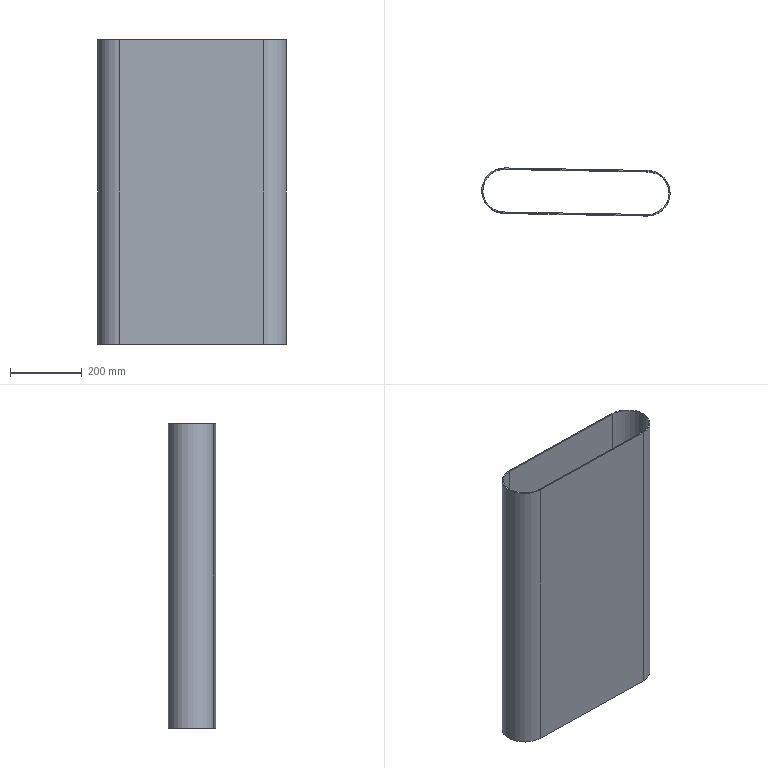Part | SolidWorks | features Extrusion 1 | 1 solid | 12 faces | box 525.939 x 132.981 x 850 mm | volume 3025361 mm3 | cylinder 6 | plane 6 | commonest cylinder face diameters 120 x3 126 x3
STEP:
#1=CARTESIAN_POINT('',(659.939,1524.019,-425.));
#2=VERTEX_POINT('',#1);
#3=CARTESIAN_POINT('',(600.986,1584.01,-425.));
#4=VERTEX_POINT('',#3);
#5=CARTESIAN_POINT('',(599.939,1524.019,-425.));
#6=DIRECTION('',(0.,0.,1.));
#7=DIRECTION('',(1.,0.,0.));
#8=AXIS2_PLACEMENT_3D('',#5,#6,#7);
#9=CIRCLE('',#8,60.);
#10=EDGE_CURVE('',#2,#4,#9,.T.);
#11=ORIENTED_EDGE('',*,*,#10,.F.);
#12=CARTESIAN_POINT('',(659.939,1524.019,425.));
#13=VERTEX_POINT('',#12);
#14=CARTESIAN_POINT('',(659.939,1524.019,-967.49));
#15=DIRECTION('',(0.,0.,1.));
#16=VECTOR('',#15,1000.);
#17=LINE('',#14,#16);
#18=EDGE_CURVE('',#2,#13,#17,.T.);
#19=ORIENTED_EDGE('',*,*,#18,.T.);
#20=CARTESIAN_POINT('',(600.986,1584.01,425.));
#21=VERTEX_POINT('',#20);
#22=CARTESIAN_POINT('',(599.939,1524.019,425.));
#23=DIRECTION('',(0.,0.,-1.));
#24=DIRECTION('',(-1.,0.,0.));
#25=AXIS2_PLACEMENT_3D('',#22,#23,#24);
#26=CIRCLE('',#25,60.);
#27=EDGE_CURVE('',#21,#13,#26,.T.);
#28=ORIENTED_EDGE('',*,*,#27,.F.);
#29=CARTESIAN_POINT('',(600.986,1584.01,-967.49));
#30=DIRECTION('',(0.,0.,1.));
#31=VECTOR('',#30,1000.);
#32=LINE('',#29,#31);
#33=EDGE_CURVE('',#4,#21,#32,.T.);
#34=ORIENTED_EDGE('',*,*,#33,.F.);
#35=EDGE_LOOP('',(#11,#19,#28,#34));
#36=FACE_OUTER_BOUND('',#35,.T.);
#37=CARTESIAN_POINT('',(599.939,1524.019,-967.49));
#38=DIRECTION('',(0.,0.,1.));
#39=DIRECTION('',(1.,0.,0.));
#40=AXIS2_PLACEMENT_3D('',#37,#38,#39);
#41=CYLINDRICAL_SURFACE('',#40,60.);
#42=ADVANCED_FACE('',(#36),#41,.F.);
#43=CARTESIAN_POINT('',(598.84,1461.029,-425.));
#44=VERTEX_POINT('',#43);
#45=CARTESIAN_POINT('',(662.939,1524.019,-425.));
#46=VERTEX_POINT('',#45);
#47=CARTESIAN_POINT('',(599.939,1524.019,-425.));
#48=DIRECTION('',(0.,0.,1.));
#49=DIRECTION('',(1.,0.,0.));
#50=AXIS2_PLACEMENT_3D('',#47,#48,#49);
#51=CIRCLE('',#50,63.);
#52=EDGE_CURVE('',#44,#46,#51,.T.);
#53=ORIENTED_EDGE('',*,*,#52,.T.);
#54=CARTESIAN_POINT('',(662.939,1524.019,425.));
#55=VERTEX_POINT('',#54);
#56=CARTESIAN_POINT('',(662.939,1524.019,-967.49));
#57=DIRECTION('',(0.,0.,1.));
#58=VECTOR('',#57,1000.);
#59=LINE('',#56,#58);
#60=EDGE_CURVE('',#46,#55,#59,.T.);
#61=ORIENTED_EDGE('',*,*,#60,.T.);
#62=CARTESIAN_POINT('',(598.84,1461.029,425.));
#63=VERTEX_POINT('',#62);
#64=CARTESIAN_POINT('',(599.939,1524.019,425.));
#65=DIRECTION('',(0.,0.,-1.));
#66=DIRECTION('',(-1.,0.,0.));
#67=AXIS2_PLACEMENT_3D('',#64,#65,#66);
#68=CIRCLE('',#67,63.);
#69=EDGE_CURVE('',#55,#63,#68,.T.);
#70=ORIENTED_EDGE('',*,*,#69,.T.);
#71=CARTESIAN_POINT('',(598.84,1461.029,-967.49));
#72=DIRECTION('',(0.,0.,1.));
#73=VECTOR('',#72,1000.);
#74=LINE('',#71,#73);
#75=EDGE_CURVE('',#44,#63,#74,.T.);
#76=ORIENTED_EDGE('',*,*,#75,.F.);
#77=EDGE_LOOP('',(#53,#61,#70,#76));
#78=FACE_OUTER_BOUND('',#77,.T.);
#79=CARTESIAN_POINT('',(599.939,1524.019,-967.49));
#80=DIRECTION('',(0.,0.,1.));
#81=DIRECTION('',(1.,0.,0.));
#82=AXIS2_PLACEMENT_3D('',#79,#80,#81);
#83=CYLINDRICAL_SURFACE('',#82,63.);
#84=ADVANCED_FACE('',(#78),#83,.T.);
#85=CARTESIAN_POINT('',(601.039,1587.009,425.));
#86=VERTEX_POINT('',#85);
#87=CARTESIAN_POINT('',(599.939,1524.019,425.));
#88=DIRECTION('',(0.,0.,-1.));
#89=DIRECTION('',(-1.,0.,0.));
#90=AXIS2_PLACEMENT_3D('',#87,#88,#89);
#91=CIRCLE('',#90,63.);
#92=EDGE_CURVE('',#86,#55,#91,.T.);
#93=ORIENTED_EDGE('',*,*,#92,.F.);
#94=CARTESIAN_POINT('',(201.1,1593.99,425.));
#95=VERTEX_POINT('',#94);
#96=CARTESIAN_POINT('',(601.039,1587.009,425.));
#97=DIRECTION('',(0.9998,-0.01745,0.));
#98=VECTOR('',#97,1000.);
#99=LINE('',#96,#98);
#100=EDGE_CURVE('',#95,#86,#99,.T.);
#101=ORIENTED_EDGE('',*,*,#100,.F.);
#102=CARTESIAN_POINT('',(198.9,1468.01,425.));
#103=VERTEX_POINT('',#102);
#104=CARTESIAN_POINT('',(200.,1531.,425.));
#105=DIRECTION('',(0.,0.,-1.));
#106=DIRECTION('',(-1.,0.,0.));
#107=AXIS2_PLACEMENT_3D('',#104,#105,#106);
#108=CIRCLE('',#107,63.);
#109=EDGE_CURVE('',#103,#95,#108,.T.);
#110=ORIENTED_EDGE('',*,*,#109,.F.);
#111=CARTESIAN_POINT('',(598.84,1461.029,425.));
#112=DIRECTION('',(-0.9998,0.01745,0.));
#113=VECTOR('',#112,1000.);
#114=LINE('',#111,#113);
#115=EDGE_CURVE('',#63,#103,#114,.T.);
#116=ORIENTED_EDGE('',*,*,#115,.F.);
#117=ORIENTED_EDGE('',*,*,#69,.F.);
#118=EDGE_LOOP('',(#93,#101,#110,#116,#117));
#119=FACE_OUTER_BOUND('',#118,.T.);
#120=ORIENTED_EDGE('',*,*,#27,.T.);
#121=CARTESIAN_POINT('',(598.892,1464.028,425.));
#122=VERTEX_POINT('',#121);
#123=CARTESIAN_POINT('',(599.939,1524.019,425.));
#124=DIRECTION('',(0.,0.,-1.));
#125=DIRECTION('',(-1.,0.,0.));
#126=AXIS2_PLACEMENT_3D('',#123,#124,#125);
#127=CIRCLE('',#126,60.);
#128=EDGE_CURVE('',#13,#122,#127,.T.);
#129=ORIENTED_EDGE('',*,*,#128,.T.);
#130=CARTESIAN_POINT('',(198.953,1471.009,425.));
#131=VERTEX_POINT('',#130);
#132=CARTESIAN_POINT('',(598.892,1464.028,425.));
#133=DIRECTION('',(-0.9998,0.01745,0.));
#134=VECTOR('',#133,1000.);
#135=LINE('',#132,#134);
#136=EDGE_CURVE('',#122,#131,#135,.T.);
#137=ORIENTED_EDGE('',*,*,#136,.T.);
#138=CARTESIAN_POINT('',(201.047,1590.991,425.));
#139=VERTEX_POINT('',#138);
#140=CARTESIAN_POINT('',(200.,1531.,425.));
#141=DIRECTION('',(0.,0.,-1.));
#142=DIRECTION('',(-1.,0.,0.));
#143=AXIS2_PLACEMENT_3D('',#140,#141,#142);
#144=CIRCLE('',#143,60.);
#145=EDGE_CURVE('',#131,#139,#144,.T.);
#146=ORIENTED_EDGE('',*,*,#145,.T.);
#147=CARTESIAN_POINT('',(600.986,1584.01,425.));
#148=DIRECTION('',(0.9998,-0.01745,0.));
#149=VECTOR('',#148,1000.);
#150=LINE('',#147,#149);
#151=EDGE_CURVE('',#139,#21,#150,.T.);
#152=ORIENTED_EDGE('',*,*,#151,.T.);
#153=EDGE_LOOP('',(#120,#129,#137,#146,#152));
#154=FACE_BOUND('',#153,.T.);
#155=CARTESIAN_POINT('',(599.939,1524.019,425.));
#156=DIRECTION('',(0.,0.,-1.));
#157=DIRECTION('',(-1.,0.,0.));
#158=AXIS2_PLACEMENT_3D('',#155,#156,#157);
#159=PLANE('',#158);
#160=ADVANCED_FACE('',(#119,#154),#159,.F.);
#161=ORIENTED_EDGE('',*,*,#60,.F.);
#162=CARTESIAN_POINT('',(601.039,1587.009,-425.));
#163=VERTEX_POINT('',#162);
#164=CARTESIAN_POINT('',(599.939,1524.019,-425.));
#165=DIRECTION('',(0.,0.,1.));
#166=DIRECTION('',(1.,0.,0.));
#167=AXIS2_PLACEMENT_3D('',#164,#165,#166);
#168=CIRCLE('',#167,63.);
#169=EDGE_CURVE('',#46,#163,#168,.T.);
#170=ORIENTED_EDGE('',*,*,#169,.T.);
#171=CARTESIAN_POINT('',(601.039,1587.009,-967.49));
#172=DIRECTION('',(0.,0.,1.));
#173=VECTOR('',#172,1000.);
#174=LINE('',#171,#173);
#175=EDGE_CURVE('',#163,#86,#174,.T.);
#176=ORIENTED_EDGE('',*,*,#175,.T.);
#177=ORIENTED_EDGE('',*,*,#92,.T.);
#178=EDGE_LOOP('',(#161,#170,#176,#177));
#179=FACE_OUTER_BOUND('',#178,.T.);
#180=CARTESIAN_POINT('',(599.939,1524.019,-967.49));
#181=DIRECTION('',(0.,0.,1.));
#182=DIRECTION('',(1.,0.,0.));
#183=AXIS2_PLACEMENT_3D('',#180,#181,#182);
#184=CYLINDRICAL_SURFACE('',#183,63.);
#185=ADVANCED_FACE('',(#179),#184,.T.);
#186=CARTESIAN_POINT('',(198.9,1468.01,-425.));
#187=VERTEX_POINT('',#186);
#188=CARTESIAN_POINT('',(198.9,1468.01,-967.49));
#189=DIRECTION('',(0.,0.,1.));
#190=VECTOR('',#189,1000.);
#191=LINE('',#188,#190);
#192=EDGE_CURVE('',#187,#103,#191,.T.);
#193=ORIENTED_EDGE('',*,*,#192,.F.);
#194=CARTESIAN_POINT('',(598.84,1461.029,-425.));
#195=DIRECTION('',(0.9998,-0.01745,0.));
#196=VECTOR('',#195,1000.);
#197=LINE('',#194,#196);
#198=EDGE_CURVE('',#187,#44,#197,.T.);
#199=ORIENTED_EDGE('',*,*,#198,.T.);
#200=ORIENTED_EDGE('',*,*,#75,.T.);
#201=ORIENTED_EDGE('',*,*,#115,.T.);
#202=EDGE_LOOP('',(#193,#199,#200,#201));
#203=FACE_OUTER_BOUND('',#202,.T.);
#204=CARTESIAN_POINT('',(598.84,1461.029,-967.49));
#205=DIRECTION('',(0.01745,0.9998,0.));
#206=DIRECTION('',(-0.9998,0.01745,0.));
#207=AXIS2_PLACEMENT_3D('',#204,#205,#206);
#208=PLANE('',#207);
#209=ADVANCED_FACE('',(#203),#208,.F.);
#210=CARTESIAN_POINT('',(201.1,1593.99,-425.));
#211=VERTEX_POINT('',#210);
#212=CARTESIAN_POINT('',(201.1,1593.99,-967.49));
#213=DIRECTION('',(0.,0.,1.));
#214=VECTOR('',#213,1000.);
#215=LINE('',#212,#214);
#216=EDGE_CURVE('',#211,#95,#215,.T.);
#217=ORIENTED_EDGE('',*,*,#216,.F.);
#218=CARTESIAN_POINT('',(200.,1531.,-425.));
#219=DIRECTION('',(0.,0.,1.));
#220=DIRECTION('',(1.,0.,0.));
#221=AXIS2_PLACEMENT_3D('',#218,#219,#220);
#222=CIRCLE('',#221,63.);
#223=EDGE_CURVE('',#211,#187,#222,.T.);
#224=ORIENTED_EDGE('',*,*,#223,.T.);
#225=ORIENTED_EDGE('',*,*,#192,.T.);
#226=ORIENTED_EDGE('',*,*,#109,.T.);
#227=EDGE_LOOP('',(#217,#224,#225,#226));
#228=FACE_OUTER_BOUND('',#227,.T.);
#229=CARTESIAN_POINT('',(200.,1531.,-967.49));
#230=DIRECTION('',(0.,0.,1.));
#231=DIRECTION('',(1.,0.,0.));
#232=AXIS2_PLACEMENT_3D('',#229,#230,#231);
#233=CYLINDRICAL_SURFACE('',#232,63.);
#234=ADVANCED_FACE('',(#228),#233,.T.);
#235=ORIENTED_EDGE('',*,*,#175,.F.);
#236=CARTESIAN_POINT('',(601.039,1587.009,-425.));
#237=DIRECTION('',(-0.9998,0.01745,0.));
#238=VECTOR('',#237,1000.);
#239=LINE('',#236,#238);
#240=EDGE_CURVE('',#163,#211,#239,.T.);
#241=ORIENTED_EDGE('',*,*,#240,.T.);
#242=ORIENTED_EDGE('',*,*,#216,.T.);
#243=ORIENTED_EDGE('',*,*,#100,.T.);
#244=EDGE_LOOP('',(#235,#241,#242,#243));
#245=FACE_OUTER_BOUND('',#244,.T.);
#246=CARTESIAN_POINT('',(601.039,1587.009,-967.49));
#247=DIRECTION('',(-0.01745,-0.9998,0.));
#248=DIRECTION('',(0.9998,-0.01745,0.));
#249=AXIS2_PLACEMENT_3D('',#246,#247,#248);
#250=PLANE('',#249);
#251=ADVANCED_FACE('',(#245),#250,.F.);
#252=ORIENTED_EDGE('',*,*,#18,.F.);
#253=CARTESIAN_POINT('',(598.892,1464.028,-425.));
#254=VERTEX_POINT('',#253);
#255=CARTESIAN_POINT('',(599.939,1524.019,-425.));
#256=DIRECTION('',(0.,0.,1.));
#257=DIRECTION('',(1.,0.,0.));
#258=AXIS2_PLACEMENT_3D('',#255,#256,#257);
#259=CIRCLE('',#258,60.);
#260=EDGE_CURVE('',#254,#2,#259,.T.);
#261=ORIENTED_EDGE('',*,*,#260,.F.);
#262=CARTESIAN_POINT('',(598.892,1464.028,-967.49));
#263=DIRECTION('',(0.,0.,1.));
#264=VECTOR('',#263,1000.);
#265=LINE('',#262,#264);
#266=EDGE_CURVE('',#254,#122,#265,.T.);
#267=ORIENTED_EDGE('',*,*,#266,.T.);
#268=ORIENTED_EDGE('',*,*,#128,.F.);
#269=EDGE_LOOP('',(#252,#261,#267,#268));
#270=FACE_OUTER_BOUND('',#269,.T.);
#271=CARTESIAN_POINT('',(599.939,1524.019,-967.49));
#272=DIRECTION('',(0.,0.,1.));
#273=DIRECTION('',(1.,0.,0.));
#274=AXIS2_PLACEMENT_3D('',#271,#272,#273);
#275=CYLINDRICAL_SURFACE('',#274,60.);
#276=ADVANCED_FACE('',(#270),#275,.F.);
#277=CARTESIAN_POINT('',(198.953,1471.009,-425.));
#278=VERTEX_POINT('',#277);
#279=CARTESIAN_POINT('',(598.892,1464.028,-425.));
#280=DIRECTION('',(0.9998,-0.01745,0.));
#281=VECTOR('',#280,1000.);
#282=LINE('',#279,#281);
#283=EDGE_CURVE('',#278,#254,#282,.T.);
#284=ORIENTED_EDGE('',*,*,#283,.F.);
#285=CARTESIAN_POINT('',(198.953,1471.009,-967.49));
#286=DIRECTION('',(0.,0.,1.));
#287=VECTOR('',#286,1000.);
#288=LINE('',#285,#287);
#289=EDGE_CURVE('',#278,#131,#288,.T.);
#290=ORIENTED_EDGE('',*,*,#289,.T.);
#291=ORIENTED_EDGE('',*,*,#136,.F.);
#292=ORIENTED_EDGE('',*,*,#266,.F.);
#293=EDGE_LOOP('',(#284,#290,#291,#292));
#294=FACE_OUTER_BOUND('',#293,.T.);
#295=CARTESIAN_POINT('',(598.892,1464.028,-967.49));
#296=DIRECTION('',(0.01745,0.9998,0.));
#297=DIRECTION('',(-0.9998,0.01745,0.));
#298=AXIS2_PLACEMENT_3D('',#295,#296,#297);
#299=PLANE('',#298);
#300=ADVANCED_FACE('',(#294),#299,.T.);
#301=CARTESIAN_POINT('',(201.047,1590.991,-425.));
#302=VERTEX_POINT('',#301);
#303=CARTESIAN_POINT('',(200.,1531.,-425.));
#304=DIRECTION('',(0.,0.,1.));
#305=DIRECTION('',(1.,0.,0.));
#306=AXIS2_PLACEMENT_3D('',#303,#304,#305);
#307=CIRCLE('',#306,60.);
#308=EDGE_CURVE('',#302,#278,#307,.T.);
#309=ORIENTED_EDGE('',*,*,#308,.F.);
#310=CARTESIAN_POINT('',(201.047,1590.991,-967.49));
#311=DIRECTION('',(0.,0.,1.));
#312=VECTOR('',#311,1000.);
#313=LINE('',#310,#312);
#314=EDGE_CURVE('',#302,#139,#313,.T.);
#315=ORIENTED_EDGE('',*,*,#314,.T.);
#316=ORIENTED_EDGE('',*,*,#145,.F.);
#317=ORIENTED_EDGE('',*,*,#289,.F.);
#318=EDGE_LOOP('',(#309,#315,#316,#317));
#319=FACE_OUTER_BOUND('',#318,.T.);
#320=CARTESIAN_POINT('',(200.,1531.,-967.49));
#321=DIRECTION('',(0.,0.,1.));
#322=DIRECTION('',(1.,0.,0.));
#323=AXIS2_PLACEMENT_3D('',#320,#321,#322);
#324=CYLINDRICAL_SURFACE('',#323,60.);
#325=ADVANCED_FACE('',(#319),#324,.F.);
#326=CARTESIAN_POINT('',(600.986,1584.01,-425.));
#327=DIRECTION('',(-0.9998,0.01745,0.));
#328=VECTOR('',#327,1000.);
#329=LINE('',#326,#328);
#330=EDGE_CURVE('',#4,#302,#329,.T.);
#331=ORIENTED_EDGE('',*,*,#330,.F.);
#332=ORIENTED_EDGE('',*,*,#33,.T.);
#333=ORIENTED_EDGE('',*,*,#151,.F.);
#334=ORIENTED_EDGE('',*,*,#314,.F.);
#335=EDGE_LOOP('',(#331,#332,#333,#334));
#336=FACE_OUTER_BOUND('',#335,.T.);
#337=CARTESIAN_POINT('',(600.986,1584.01,-967.49));
#338=DIRECTION('',(-0.01745,-0.9998,0.));
#339=DIRECTION('',(0.9998,-0.01745,0.));
#340=AXIS2_PLACEMENT_3D('',#337,#338,#339);
#341=PLANE('',#340);
#342=ADVANCED_FACE('',(#336),#341,.T.);
#343=ORIENTED_EDGE('',*,*,#260,.T.);
#344=ORIENTED_EDGE('',*,*,#10,.T.);
#345=ORIENTED_EDGE('',*,*,#330,.T.);
#346=ORIENTED_EDGE('',*,*,#308,.T.);
#347=ORIENTED_EDGE('',*,*,#283,.T.);
#348=EDGE_LOOP('',(#343,#344,#345,#346,#347));
#349=FACE_BOUND('',#348,.T.);
#350=ORIENTED_EDGE('',*,*,#198,.F.);
#351=ORIENTED_EDGE('',*,*,#223,.F.);
#352=ORIENTED_EDGE('',*,*,#240,.F.);
#353=ORIENTED_EDGE('',*,*,#169,.F.);
#354=ORIENTED_EDGE('',*,*,#52,.F.);
#355=EDGE_LOOP('',(#350,#351,#352,#353,#354));
#356=FACE_OUTER_BOUND('',#355,.T.);
#357=CARTESIAN_POINT('',(200.,1591.,-425.));
#358=DIRECTION('',(0.,0.,1.));
#359=DIRECTION('',(1.,0.,0.));
#360=AXIS2_PLACEMENT_3D('',#357,#358,#359);
#361=PLANE('',#360);
#362=ADVANCED_FACE('',(#349,#356),#361,.F.);
#363=CLOSED_SHELL('',(#42,#84,#160,#185,#209,#234,#251,#276,#300,#325,#342,#362));
#364=MANIFOLD_SOLID_BREP('',#363);
#365=CARTESIAN_POINT('',(0.,0.,0.));
#366=DIRECTION('',(0.,0.,1.));
#367=DIRECTION('',(1.,0.,0.));
#368=AXIS2_PLACEMENT_3D('',#365,#366,#367);
#369=(LENGTH_UNIT()NAMED_UNIT(*)SI_UNIT(.MILLI.,.METRE.));
#370=UNCERTAINTY_MEASURE_WITH_UNIT(LENGTH_MEASURE(0.00001),#369,'','');
#371=(NAMED_UNIT(*)PLANE_ANGLE_UNIT()SI_UNIT($,.RADIAN.));
#372=(NAMED_UNIT(*)SI_UNIT($,.STERADIAN.)SOLID_ANGLE_UNIT());
#373=(GEOMETRIC_REPRESENTATION_CONTEXT(3)GLOBAL_UNCERTAINTY_ASSIGNED_CONTEXT((#370))GLOBAL_UNIT_ASSIGNED_CONTEXT((#369,#371,#372))REPRESENTATION_CONTEXT('',''));
#374=ADVANCED_BREP_SHAPE_REPRESENTATION('',(#364,#368),#373);